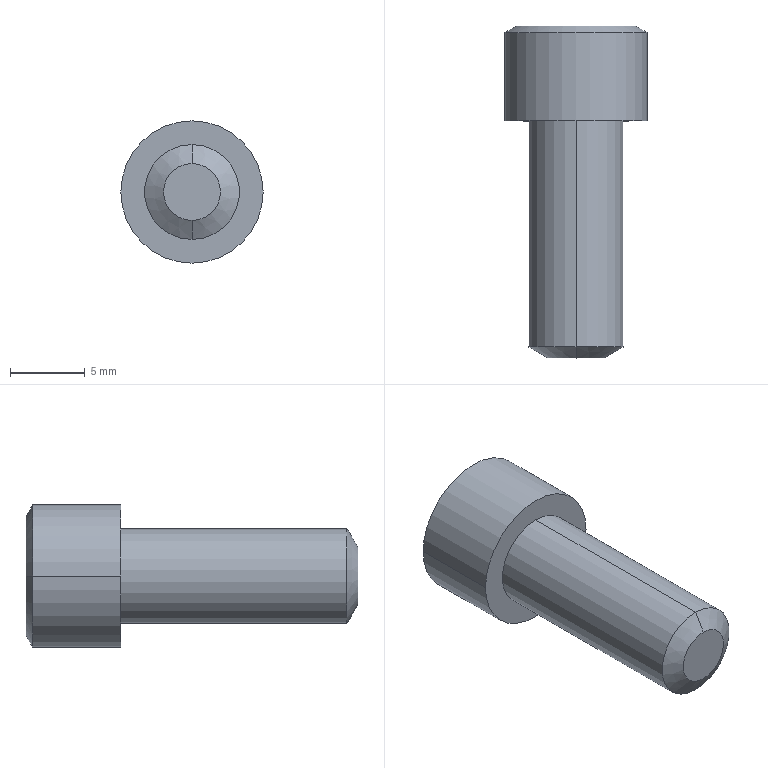Part | NX | features BREP 1 | 1 solid | 11 faces | box 9.525 x 22.225 x 9.525 mm | volume 942.425 mm3 | cone 4 | cylinder 4 | plane 3 | commonest cylinder face diameters 6.35 x2 9.525 x2
STEP:
#1=CARTESIAN_POINT('',(0.,-15.875,1.905));
#2=VERTEX_POINT('',#1);
#3=CARTESIAN_POINT('',(0.,-15.875,-1.905));
#4=VERTEX_POINT('',#3);
#5=CARTESIAN_POINT('',(0.,-15.875,0.));
#6=DIRECTION('',(0.,-1.,0.));
#7=DIRECTION('',(0.,0.,1.));
#8=AXIS2_PLACEMENT_3D('',#5,#6,#7);
#9=CIRCLE('',#8,1.905);
#10=EDGE_CURVE('',#2,#4,#9,.T.);
#11=ORIENTED_EDGE('',*,*,#10,.T.);
#12=CARTESIAN_POINT('',(0.,-15.875,0.));
#13=DIRECTION('',(0.,-1.,0.));
#14=DIRECTION('',(0.,0.,-1.));
#15=AXIS2_PLACEMENT_3D('',#12,#13,#14);
#16=CIRCLE('',#15,1.905);
#17=EDGE_CURVE('',#4,#2,#16,.T.);
#18=ORIENTED_EDGE('',*,*,#17,.T.);
#19=EDGE_LOOP('',(#11,#18));
#20=FACE_BOUND('',#19,.T.);
#21=CARTESIAN_POINT('',(0.,-15.875,0.));
#22=DIRECTION('',(0.,-1.,0.));
#23=DIRECTION('',(0.,0.,-1.));
#24=AXIS2_PLACEMENT_3D('',#21,#22,#23);
#25=PLANE('',#24);
#26=ADVANCED_FACE('',(#20),#25,.T.);
#27=CARTESIAN_POINT('',(0.,-15.142,-3.175));
#28=VERTEX_POINT('',#27);
#29=CARTESIAN_POINT('',(0.,-15.875,-1.905));
#30=DIRECTION('',(0.,0.5,-0.866));
#31=VECTOR('',#30,1000.);
#32=LINE('',#29,#31);
#33=EDGE_CURVE('',#4,#28,#32,.T.);
#34=ORIENTED_EDGE('',*,*,#33,.T.);
#35=CARTESIAN_POINT('',(0.,-15.142,3.175));
#36=VERTEX_POINT('',#35);
#37=CARTESIAN_POINT('',(0.,-15.142,0.));
#38=DIRECTION('',(0.,-1.,0.));
#39=DIRECTION('',(0.,0.,-1.));
#40=AXIS2_PLACEMENT_3D('',#37,#38,#39);
#41=CIRCLE('',#40,3.175);
#42=EDGE_CURVE('',#28,#36,#41,.T.);
#43=ORIENTED_EDGE('',*,*,#42,.T.);
#44=CARTESIAN_POINT('',(0.,-15.875,1.905));
#45=DIRECTION('',(0.,0.5,0.866));
#46=VECTOR('',#45,1000.);
#47=LINE('',#44,#46);
#48=EDGE_CURVE('',#2,#36,#47,.T.);
#49=ORIENTED_EDGE('',*,*,#48,.F.);
#50=ORIENTED_EDGE('',*,*,#17,.F.);
#51=EDGE_LOOP('',(#34,#43,#49,#50));
#52=FACE_BOUND('',#51,.T.);
#53=CARTESIAN_POINT('',(0.,-15.508,0.));
#54=DIRECTION('',(0.,1.,0.));
#55=DIRECTION('',(0.,0.,1.));
#56=AXIS2_PLACEMENT_3D('',#53,#54,#55);
#57=CONICAL_SURFACE('',#56,2.54,1.047);
#58=ADVANCED_FACE('',(#52),#57,.T.);
#59=ORIENTED_EDGE('',*,*,#48,.T.);
#60=CARTESIAN_POINT('',(0.,-15.142,0.));
#61=DIRECTION('',(0.,-1.,0.));
#62=DIRECTION('',(0.,0.,1.));
#63=AXIS2_PLACEMENT_3D('',#60,#61,#62);
#64=CIRCLE('',#63,3.175);
#65=EDGE_CURVE('',#36,#28,#64,.T.);
#66=ORIENTED_EDGE('',*,*,#65,.T.);
#67=ORIENTED_EDGE('',*,*,#33,.F.);
#68=ORIENTED_EDGE('',*,*,#10,.F.);
#69=EDGE_LOOP('',(#59,#66,#67,#68));
#70=FACE_BOUND('',#69,.T.);
#71=CARTESIAN_POINT('',(0.,-15.508,0.));
#72=DIRECTION('',(0.,1.,0.));
#73=DIRECTION('',(0.,0.,1.));
#74=AXIS2_PLACEMENT_3D('',#71,#72,#73);
#75=CONICAL_SURFACE('',#74,2.54,1.047);
#76=ADVANCED_FACE('',(#70),#75,.T.);
#77=CARTESIAN_POINT('',(0.,0.,-3.175));
#78=VERTEX_POINT('',#77);
#79=CARTESIAN_POINT('',(0.,0.,-3.175));
#80=DIRECTION('',(0.,-1.,0.));
#81=VECTOR('',#80,1000.);
#82=LINE('',#79,#81);
#83=EDGE_CURVE('',#78,#28,#82,.T.);
#84=ORIENTED_EDGE('',*,*,#83,.T.);
#85=ORIENTED_EDGE('',*,*,#65,.F.);
#86=CARTESIAN_POINT('',(0.,0.,3.175));
#87=VERTEX_POINT('',#86);
#88=CARTESIAN_POINT('',(0.,0.,3.175));
#89=DIRECTION('',(0.,-1.,0.));
#90=VECTOR('',#89,1000.);
#91=LINE('',#88,#90);
#92=EDGE_CURVE('',#87,#36,#91,.T.);
#93=ORIENTED_EDGE('',*,*,#92,.F.);
#94=CARTESIAN_POINT('',(0.,0.,0.));
#95=DIRECTION('',(0.,-1.,0.));
#96=DIRECTION('',(0.,0.,1.));
#97=AXIS2_PLACEMENT_3D('',#94,#95,#96);
#98=CIRCLE('',#97,3.175);
#99=EDGE_CURVE('',#87,#78,#98,.T.);
#100=ORIENTED_EDGE('',*,*,#99,.T.);
#101=EDGE_LOOP('',(#84,#85,#93,#100));
#102=FACE_BOUND('',#101,.T.);
#103=CARTESIAN_POINT('',(0.,0.,0.));
#104=DIRECTION('',(0.,-1.,0.));
#105=DIRECTION('',(0.,0.,-1.));
#106=AXIS2_PLACEMENT_3D('',#103,#104,#105);
#107=CYLINDRICAL_SURFACE('',#106,3.175);
#108=ADVANCED_FACE('',(#102),#107,.T.);
#109=CARTESIAN_POINT('',(-4.763,0.,0.));
#110=VERTEX_POINT('',#109);
#111=CARTESIAN_POINT('',(4.763,0.,0.));
#112=VERTEX_POINT('',#111);
#113=CARTESIAN_POINT('',(0.,0.,0.));
#114=DIRECTION('',(0.,1.,0.));
#115=DIRECTION('',(-1.,0.,0.));
#116=AXIS2_PLACEMENT_3D('',#113,#114,#115);
#117=CIRCLE('',#116,4.763);
#118=EDGE_CURVE('',#110,#112,#117,.T.);
#119=ORIENTED_EDGE('',*,*,#118,.F.);
#120=CARTESIAN_POINT('',(0.,0.,0.));
#121=DIRECTION('',(0.,1.,0.));
#122=DIRECTION('',(1.,0.,0.));
#123=AXIS2_PLACEMENT_3D('',#120,#121,#122);
#124=CIRCLE('',#123,4.763);
#125=EDGE_CURVE('',#112,#110,#124,.T.);
#126=ORIENTED_EDGE('',*,*,#125,.F.);
#127=EDGE_LOOP('',(#119,#126));
#128=FACE_BOUND('',#127,.T.);
#129=ORIENTED_EDGE('',*,*,#99,.F.);
#130=CARTESIAN_POINT('',(0.,0.,0.));
#131=DIRECTION('',(0.,-1.,0.));
#132=DIRECTION('',(0.,0.,-1.));
#133=AXIS2_PLACEMENT_3D('',#130,#131,#132);
#134=CIRCLE('',#133,3.175);
#135=EDGE_CURVE('',#78,#87,#134,.T.);
#136=ORIENTED_EDGE('',*,*,#135,.F.);
#137=EDGE_LOOP('',(#129,#136));
#138=FACE_BOUND('',#137,.T.);
#139=CARTESIAN_POINT('',(0.,0.,0.));
#140=DIRECTION('',(0.,1.,0.));
#141=DIRECTION('',(1.,0.,0.));
#142=AXIS2_PLACEMENT_3D('',#139,#140,#141);
#143=PLANE('',#142);
#144=ADVANCED_FACE('',(#128,#138),#143,.F.);
#145=CARTESIAN_POINT('',(-4.763,5.91,0.));
#146=VERTEX_POINT('',#145);
#147=CARTESIAN_POINT('',(-4.763,0.,0.));
#148=DIRECTION('',(0.,1.,0.));
#149=VECTOR('',#148,1000.);
#150=LINE('',#147,#149);
#151=EDGE_CURVE('',#110,#146,#150,.T.);
#152=ORIENTED_EDGE('',*,*,#151,.T.);
#153=CARTESIAN_POINT('',(4.763,5.91,0.));
#154=VERTEX_POINT('',#153);
#155=CARTESIAN_POINT('',(0.,5.91,0.));
#156=DIRECTION('',(0.,1.,0.));
#157=DIRECTION('',(1.,0.,0.));
#158=AXIS2_PLACEMENT_3D('',#155,#156,#157);
#159=CIRCLE('',#158,4.763);
#160=EDGE_CURVE('',#154,#146,#159,.T.);
#161=ORIENTED_EDGE('',*,*,#160,.F.);
#162=CARTESIAN_POINT('',(4.763,0.,0.));
#163=DIRECTION('',(0.,1.,0.));
#164=VECTOR('',#163,1000.);
#165=LINE('',#162,#164);
#166=EDGE_CURVE('',#112,#154,#165,.T.);
#167=ORIENTED_EDGE('',*,*,#166,.F.);
#168=ORIENTED_EDGE('',*,*,#125,.T.);
#169=EDGE_LOOP('',(#152,#161,#167,#168));
#170=FACE_BOUND('',#169,.T.);
#171=CARTESIAN_POINT('',(0.,0.,0.));
#172=DIRECTION('',(0.,1.,0.));
#173=DIRECTION('',(1.,0.,0.));
#174=AXIS2_PLACEMENT_3D('',#171,#172,#173);
#175=CYLINDRICAL_SURFACE('',#174,4.763);
#176=ADVANCED_FACE('',(#170),#175,.T.);
#177=ORIENTED_EDGE('',*,*,#166,.T.);
#178=CARTESIAN_POINT('',(0.,5.91,0.));
#179=DIRECTION('',(0.,1.,0.));
#180=DIRECTION('',(-1.,0.,0.));
#181=AXIS2_PLACEMENT_3D('',#178,#179,#180);
#182=CIRCLE('',#181,4.763);
#183=EDGE_CURVE('',#146,#154,#182,.T.);
#184=ORIENTED_EDGE('',*,*,#183,.F.);
#185=ORIENTED_EDGE('',*,*,#151,.F.);
#186=ORIENTED_EDGE('',*,*,#118,.T.);
#187=EDGE_LOOP('',(#177,#184,#185,#186));
#188=FACE_BOUND('',#187,.T.);
#189=CARTESIAN_POINT('',(0.,0.,0.));
#190=DIRECTION('',(0.,1.,0.));
#191=DIRECTION('',(1.,0.,0.));
#192=AXIS2_PLACEMENT_3D('',#189,#190,#191);
#193=CYLINDRICAL_SURFACE('',#192,4.763);
#194=ADVANCED_FACE('',(#188),#193,.T.);
#195=CARTESIAN_POINT('',(-4.,6.35,0.));
#196=VERTEX_POINT('',#195);
#197=CARTESIAN_POINT('',(-4.,6.35,0.));
#198=DIRECTION('',(-0.866,-0.5,0.));
#199=VECTOR('',#198,1000.);
#200=LINE('',#197,#199);
#201=EDGE_CURVE('',#196,#146,#200,.T.);
#202=ORIENTED_EDGE('',*,*,#201,.T.);
#203=ORIENTED_EDGE('',*,*,#183,.T.);
#204=CARTESIAN_POINT('',(4.,6.35,0.));
#205=VERTEX_POINT('',#204);
#206=CARTESIAN_POINT('',(4.,6.35,0.));
#207=DIRECTION('',(0.866,-0.5,0.));
#208=VECTOR('',#207,1000.);
#209=LINE('',#206,#208);
#210=EDGE_CURVE('',#205,#154,#209,.T.);
#211=ORIENTED_EDGE('',*,*,#210,.F.);
#212=CARTESIAN_POINT('',(0.,6.35,0.));
#213=DIRECTION('',(0.,1.,0.));
#214=DIRECTION('',(-1.,0.,0.));
#215=AXIS2_PLACEMENT_3D('',#212,#213,#214);
#216=CIRCLE('',#215,4.);
#217=EDGE_CURVE('',#196,#205,#216,.T.);
#218=ORIENTED_EDGE('',*,*,#217,.F.);
#219=EDGE_LOOP('',(#202,#203,#211,#218));
#220=FACE_BOUND('',#219,.T.);
#221=CARTESIAN_POINT('',(0.,6.13,0.));
#222=DIRECTION('',(0.,-1.,0.));
#223=DIRECTION('',(-1.,0.,0.));
#224=AXIS2_PLACEMENT_3D('',#221,#222,#223);
#225=CONICAL_SURFACE('',#224,4.381,1.047);
#226=ADVANCED_FACE('',(#220),#225,.T.);
#227=ORIENTED_EDGE('',*,*,#217,.T.);
#228=CARTESIAN_POINT('',(0.,6.35,0.));
#229=DIRECTION('',(0.,1.,0.));
#230=DIRECTION('',(1.,0.,0.));
#231=AXIS2_PLACEMENT_3D('',#228,#229,#230);
#232=CIRCLE('',#231,4.);
#233=EDGE_CURVE('',#205,#196,#232,.T.);
#234=ORIENTED_EDGE('',*,*,#233,.T.);
#235=EDGE_LOOP('',(#227,#234));
#236=FACE_BOUND('',#235,.T.);
#237=CARTESIAN_POINT('',(0.,6.35,0.));
#238=DIRECTION('',(0.,1.,0.));
#239=DIRECTION('',(1.,0.,0.));
#240=AXIS2_PLACEMENT_3D('',#237,#238,#239);
#241=PLANE('',#240);
#242=ADVANCED_FACE('',(#236),#241,.T.);
#243=ORIENTED_EDGE('',*,*,#210,.T.);
#244=ORIENTED_EDGE('',*,*,#160,.T.);
#245=ORIENTED_EDGE('',*,*,#201,.F.);
#246=ORIENTED_EDGE('',*,*,#233,.F.);
#247=EDGE_LOOP('',(#243,#244,#245,#246));
#248=FACE_BOUND('',#247,.T.);
#249=CARTESIAN_POINT('',(0.,6.13,0.));
#250=DIRECTION('',(0.,-1.,0.));
#251=DIRECTION('',(-1.,0.,0.));
#252=AXIS2_PLACEMENT_3D('',#249,#250,#251);
#253=CONICAL_SURFACE('',#252,4.381,1.047);
#254=ADVANCED_FACE('',(#248),#253,.T.);
#255=ORIENTED_EDGE('',*,*,#92,.T.);
#256=ORIENTED_EDGE('',*,*,#42,.F.);
#257=ORIENTED_EDGE('',*,*,#83,.F.);
#258=ORIENTED_EDGE('',*,*,#135,.T.);
#259=EDGE_LOOP('',(#255,#256,#257,#258));
#260=FACE_BOUND('',#259,.T.);
#261=CARTESIAN_POINT('',(0.,0.,0.));
#262=DIRECTION('',(0.,-1.,0.));
#263=DIRECTION('',(0.,0.,-1.));
#264=AXIS2_PLACEMENT_3D('',#261,#262,#263);
#265=CYLINDRICAL_SURFACE('',#264,3.175);
#266=ADVANCED_FACE('',(#260),#265,.T.);
#267=CLOSED_SHELL('',(#26,#58,#76,#108,#144,#176,#194,#226,#242,#254,#266));
#268=MANIFOLD_SOLID_BREP('',#267);
#269=(LENGTH_UNIT()NAMED_UNIT(*)SI_UNIT(.MILLI.,.METRE.));
#270=UNCERTAINTY_MEASURE_WITH_UNIT(LENGTH_MEASURE(0.00001),#269,'','');
#271=(NAMED_UNIT(*)PLANE_ANGLE_UNIT()SI_UNIT($,.RADIAN.));
#272=(NAMED_UNIT(*)SI_UNIT($,.STERADIAN.)SOLID_ANGLE_UNIT());
#273=(GEOMETRIC_REPRESENTATION_CONTEXT(3)GLOBAL_UNCERTAINTY_ASSIGNED_CONTEXT((#270))GLOBAL_UNIT_ASSIGNED_CONTEXT((#269,#271,#272))REPRESENTATION_CONTEXT('',''));
#274=ADVANCED_BREP_SHAPE_REPRESENTATION('',(#268),#273);